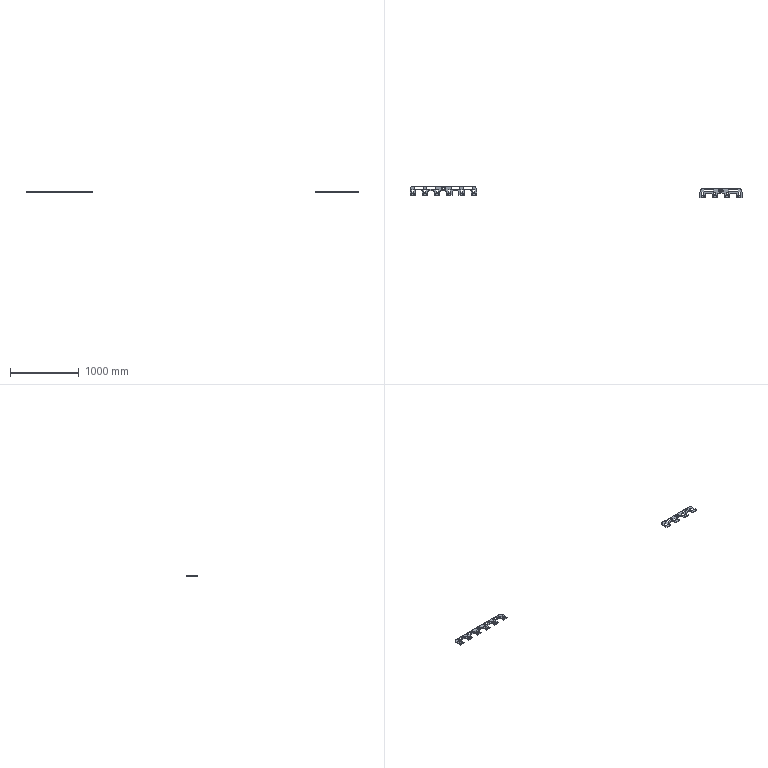NC program | NX | posted with a generic post | part box 4825 x 168.213 x 13 mm
Lines 1366 to 2532 of 4378:
(ZLEVEL_PROFILE_COPY_1_COPY_COPY , TOOL : D6)
N2688 T06 M6
N2690 G54
N2692 G17 G0 G90 X414.221 Y-3.8 S9500 M3
N2694 G43 Z30. H6
N2696 Z-0.591
N2698 G94 G1 Y-4.997 F1000.
N2700 X414.284 Y-5.
N2702 X416.5 F1650.
N2704 Y-2.784
N2706 X416.497 Y-2.721
N2708 X415.3
N2710 G0 X414.221 Y-3.8 Z-1.182
N2712 G1 Y-4.997 F1000.
N2714 X414.284 Y-5.
N2716 X416.5 F1650.
N2718 Y-2.784
N2720 X416.497 Y-2.721
N2722 X415.3
N2724 G0 X414.221 Y-3.8 Z-1.773
N2726 G1 Y-4.997 F1000.
N2728 X414.284 Y-5.
N2730 X416.5 F1650.
N2732 Y-2.784
N2734 X416.497 Y-2.721
N2736 X415.3
N2738 G0 X414.221 Y-3.8 Z-2.364
N2740 G1 Y-4.997 F1000.
N2742 X414.284 Y-5.
N2744 X416.5 F1650.
N2746 Y-2.784
N2748 X416.497 Y-2.721
N2750 X415.3
N2752 G0 X414.221 Y-3.8 Z-2.955
N2754 G1 Y-4.997 F1000.
N2756 X414.284 Y-5.
N2758 X416.5 F1650.
N2760 Y-2.784
N2762 X416.497 Y-2.721
N2764 X415.3
N2766 G0 X414.221 Y-3.8 Z-3.545
N2768 G1 Y-4.997 F1000.
N2770 X414.284 Y-5.
N2772 X416.5 F1650.
N2774 Y-2.784
N2776 X416.497 Y-2.721
N2778 X415.3
N2780 G0 X414.221 Y-3.8 Z-4.136
N2782 G1 Y-4.997 F1000.
N2784 X414.284 Y-5.
N2786 X416.5 F1650.
N2788 Y-2.784
N2790 X416.497 Y-2.721
N2792 X415.3
N2794 G0 X414.221 Y-3.8 Z-4.727
N2796 G1 Y-4.997 F1000.
N2798 X414.284 Y-5.
N2800 X416.5 F1650.
N2802 Y-2.784
N2804 X416.497 Y-2.721
N2806 X415.3
N2808 G0 X414.221 Y-3.8 Z-5.318
N2810 G1 Y-4.997 F1000.
N2812 X414.284 Y-5.
N2814 X416.5 F1650.
N2816 Y-2.784
N2818 X416.497 Y-2.721
N2820 X415.3
N2822 G0 X414.221 Y-3.8 Z-5.909
N2824 G1 Y-4.997 F1000.
N2826 X414.284 Y-5.
N2828 X416.5 F1650.
N2830 Y-2.784
N2832 X416.497 Y-2.721
N2834 X415.3
N2836 G0 X414.221 Y-3.8 Z-6.5
N2838 G1 Y-4.997 F1000.
N2840 X414.284 Y-5.
N2842 X416.5 F1650.
N2844 Y-2.784
N2846 X416.497 Y-2.721
N2848 X415.3
N2850 G0 X414.221 Y-3.8 Z-7.091
N2852 G1 Y-4.997 F1000.
N2854 X414.284 Y-5.
N2856 X416.5 F1650.
N2858 Y-2.784
N2860 X416.497 Y-2.721
N2862 X415.3
N2864 G0 X414.221 Y-3.8 Z-7.682
N2866 G1 Y-4.997 F1000.
N2868 X414.284 Y-5.
N2870 X416.5 F1650.
N2872 Y-2.784
N2874 X416.497 Y-2.721
N2876 X415.3
N2878 G0 X414.211 Y-3.8 Z-8.273
N2880 G1 Y-4.997 F1000.
N2882 X414.273 Y-5.
N2884 X416.5 F1650.
N2886 Y-2.782
N2888 X416.497 Y-2.719
N2890 X415.3
N2892 G0 X414.211 Y-3.8 Z-8.864
N2894 G1 Y-4.997 F1000.
N2896 X414.273 Y-5.
N2898 X416.5 F1650.
N2900 Y-2.782
N2902 X416.497 Y-2.719
N2904 X415.3
N2906 G0 X414.211 Y-3.8 Z-9.455
N2908 G1 Y-4.997 F1000.
N2910 X414.273 Y-5.
N2912 X416.5 F1650.
N2914 Y-2.782
N2916 X416.497 Y-2.719
N2918 X415.3
N2920 G0 X414.211 Y-3.8 Z-10.045
N2922 G1 Y-4.997 F1000.
N2924 X414.273 Y-5.
N2926 X416.5 F1650.
N2928 Y-2.782
N2930 X416.497 Y-2.719
N2932 X415.3
N2934 G0 X414.211 Y-3.8 Z-10.636
N2936 G1 Y-4.997 F1000.
N2938 X414.273 Y-5.
N2940 X416.5 F1650.
N2942 Y-2.782
N2944 X416.497 Y-2.719
N2946 X415.3
N2948 G0 X414.211 Y-3.8 Z-11.227
N2950 G1 Y-4.997 F1000.
N2952 X414.273 Y-5.
N2954 X416.5 F1650.
N2956 Y-2.782
N2958 X416.497 Y-2.719
N2960 X415.3
N2962 G0 X414.211 Y-3.8 Z-11.818
N2964 G1 Y-4.997 F1000.
N2966 X414.273 Y-5.
N2968 X416.5 F1650.
N2970 Y-2.782
N2972 X416.497 Y-2.719
N2974 X415.3
N2976 G0 X414.211 Y-3.8 Z-12.409
N2978 G1 Y-4.997 F1000.
N2980 X414.273 Y-5.
N2982 X416.5 F1650.
N2984 Y-2.782
N2986 X416.497 Y-2.719
N2988 X415.3
N2990 G0 X414.211 Y-3.8 Z-13.
N2992 G1 Y-4.997 F1000.
N2994 X414.273 Y-5.
N2996 X416.5 F1650.
N2998 Y-2.782
N3000 X416.497 Y-2.719
N3002 X415.3
N3004 G0 Z30.
N3006 Y18.721
N3008 Z-0.591
N3010 G1 X416.497 F1000.
N3012 X416.5 Y18.784
N3014 Y21. F1650.
N3016 X414.284
N3018 X414.221 Y20.997
N3020 Y19.8
N3022 G0 X415.3 Y18.721 Z-1.182
N3024 G1 X416.497 F1000.
N3026 X416.5 Y18.784
N3028 Y21. F1650.
N3030 X414.284
N3032 X414.221 Y20.997
N3034 Y19.8
N3036 G0 X415.3 Y18.721 Z-1.773
N3038 G1 X416.497 F1000.
N3040 X416.5 Y18.784
N3042 Y21. F1650.
N3044 X414.284
N3046 X414.221 Y20.997
N3048 Y19.8
N3050 G0 X415.3 Y18.721 Z-2.364
N3052 G1 X416.497 F1000.
N3054 X416.5 Y18.784
N3056 Y21. F1650.
N3058 X414.284
N3060 X414.221 Y20.997
N3062 Y19.8
N3064 G0 X415.3 Y18.721 Z-2.955
N3066 G1 X416.497 F1000.
N3068 X416.5 Y18.784
N3070 Y21. F1650.
N3072 X414.284
N3074 X414.221 Y20.997
N3076 Y19.8
N3078 G0 X415.3 Y18.721 Z-3.545
N3080 G1 X416.497 F1000.
N3082 X416.5 Y18.784
N3084 Y21. F1650.
N3086 X414.284
N3088 X414.221 Y20.997
N3090 Y19.8
N3092 G0 X415.3 Y18.721 Z-4.136
N3094 G1 X416.497 F1000.
N3096 X416.5 Y18.784
N3098 Y21. F1650.
N3100 X414.284
N3102 X414.221 Y20.997
N3104 Y19.8
N3106 G0 X415.3 Y18.721 Z-4.727
N3108 G1 X416.497 F1000.
N3110 X416.5 Y18.784
N3112 Y21. F1650.
N3114 X414.284
N3116 X414.221 Y20.997
N3118 Y19.8
N3120 G0 X415.3 Y18.721 Z-5.318
N3122 G1 X416.497 F1000.
N3124 X416.5 Y18.784
N3126 Y21. F1650.
N3128 X414.284
N3130 X414.221 Y20.997
N3132 Y19.8
N3134 G0 X415.3 Y18.721 Z-5.909
N3136 G1 X416.497 F1000.
N3138 X416.5 Y18.784
N3140 Y21. F1650.
N3142 X414.284
N3144 X414.221 Y20.997
N3146 Y19.8
N3148 G0 X415.3 Y18.721 Z-6.5
N3150 G1 X416.497 F1000.
N3152 X416.5 Y18.784
N3154 Y21. F1650.
N3156 X414.284
N3158 X414.221 Y20.997
N3160 Y19.8
N3162 G0 X415.3 Y18.721 Z-7.091
N3164 G1 X416.497 F1000.
N3166 X416.5 Y18.784
N3168 Y21. F1650.
N3170 X414.284
N3172 X414.221 Y20.997
N3174 Y19.8
N3176 G0 X415.3 Y18.721 Z-7.682
N3178 G1 X416.497 F1000.
N3180 X416.5 Y18.784
N3182 Y21. F1650.
N3184 X414.284
N3186 X414.221 Y20.997
N3188 Y19.8
N3190 G0 X415.3 Y18.729 Z-8.273
N3192 G1 X416.497 F1000.
N3194 X416.5 Y18.792
N3196 Y20.988 F1650.
N3198 Y21.
N3200 X414.292
N3202 X414.229 Y20.997
N3204 Y19.8
N3206 G0 X415.3 Y18.729 Z-8.864
N3208 G1 X416.497 F1000.
N3210 X416.5 Y18.792
N3212 Y20.988 F1650.
N3214 Y21.
N3216 X414.292
N3218 X414.229 Y20.997
N3220 Y19.8
N3222 G0 X415.3 Y18.729 Z-9.455
N3224 G1 X416.497 F1000.
N3226 X416.5 Y18.792
N3228 Y20.988 F1650.
N3230 Y21.
N3232 X414.292
N3234 X414.229 Y20.997
N3236 Y19.8
N3238 G0 X415.3 Y18.729 Z-10.045
N3240 G1 X416.497 F1000.
N3242 X416.5 Y18.792
N3244 Y20.988 F1650.
N3246 Y21.
N3248 X414.292
N3250 X414.229 Y20.997
N3252 Y19.8
N3254 G0 X415.3 Y18.729 Z-10.636
N3256 G1 X416.497 F1000.
N3258 X416.5 Y18.792
N3260 Y20.988 F1650.
N3262 Y21.
N3264 X414.292
N3266 X414.229 Y20.997
N3268 Y19.8
N3270 G0 X415.3 Y18.729 Z-11.227
N3272 G1 X416.497 F1000.
N3274 X416.5 Y18.792
N3276 Y20.988 F1650.
N3278 Y21.
N3280 X414.292
N3282 X414.229 Y20.997
N3284 Y19.8
N3286 G0 X415.3 Y18.729 Z-11.818
N3288 G1 X416.497 F1000.
N3290 X416.5 Y18.792
N3292 Y20.988 F1650.
N3294 Y21.
N3296 X414.292
N3298 X414.229 Y20.997
N3300 Y19.8
N3302 G0 X415.3 Y18.729 Z-12.409
N3304 G1 X416.497 F1000.
N3306 X416.5 Y18.792
N3308 Y20.988 F1650.
N3310 Y21.
N3312 X414.292
N3314 X414.229 Y20.997
N3316 Y19.8
N3318 G0 X415.3 Y18.729 Z-13.
N3320 G1 X416.497 F1000.
N3322 X416.5 Y18.792
N3324 Y20.988 F1650.
N3326 Y21.
N3328 X414.292
N3330 X414.229 Y20.997
N3332 Y19.8
N3334 G0 Z30.
N3336 X296.979
N3338 Z-0.591
N3340 G1 Y20.997 F1000.
N3342 X296.916 Y21.
N3344 X294.7 F1650.
N3346 Y18.784
N3348 X294.703 Y18.721
N3350 X295.9
N3352 G0 X296.979 Y19.8 Z-1.182
N3354 G1 Y20.997 F1000.
N3356 X296.916 Y21.
N3358 X294.7 F1650.
N3360 Y18.784
N3362 X294.703 Y18.721
N3364 X295.9
N3366 G0 X296.979 Y19.8 Z-1.773
N3368 G1 Y20.997 F1000.
N3370 X296.916 Y21.
N3372 X294.7 F1650.
N3374 Y18.784
N3376 X294.703 Y18.721
N3378 X295.9
N3380 G0 X296.979 Y19.8 Z-2.364
N3382 G1 Y20.997 F1000.
N3384 X296.916 Y21.
N3386 X294.7 F1650.
N3388 Y18.784
N3390 X294.703 Y18.721
N3392 X295.9
N3394 G0 X296.979 Y19.8 Z-2.955
N3396 G1 Y20.997 F1000.
N3398 X296.916 Y21.
N3400 X294.7 F1650.
N3402 Y18.784
N3404 X294.703 Y18.721
N3406 X295.9
N3408 G0 X296.979 Y19.8 Z-3.545
N3410 G1 Y20.997 F1000.
N3412 X296.916 Y21.
N3414 X294.7 F1650.
N3416 Y18.784
N3418 X294.703 Y18.721
N3420 X295.9
N3422 G0 X296.979 Y19.8 Z-4.136
N3424 G1 Y20.997 F1000.
N3426 X296.916 Y21.
N3428 X294.7 F1650.
N3430 Y18.784
N3432 X294.703 Y18.721
N3434 X295.9
N3436 G0 X296.979 Y19.8 Z-4.727
N3438 G1 Y20.997 F1000.
N3440 X296.916 Y21.
N3442 X294.7 F1650.
N3444 Y18.784
N3446 X294.703 Y18.721
N3448 X295.9
N3450 G0 X296.979 Y19.8 Z-5.318
N3452 G1 Y20.997 F1000.
N3454 X296.916 Y21.
N3456 X294.7 F1650.
N3458 Y18.784
N3460 X294.703 Y18.721
N3462 X295.9
N3464 G0 X296.979 Y19.8 Z-5.909
N3466 G1 Y20.997 F1000.
N3468 X296.916 Y21.
N3470 X294.7 F1650.
N3472 Y18.784
N3474 X294.703 Y18.721
N3476 X295.9
N3478 G0 X296.979 Y19.8 Z-6.5
N3480 G1 Y20.997 F1000.
N3482 X296.916 Y21.
N3484 X294.7 F1650.
N3486 Y18.784
N3488 X294.703 Y18.721
N3490 X295.9
N3492 G0 X296.979 Y19.8 Z-7.091
N3494 G1 Y20.997 F1000.
N3496 X296.916 Y21.
N3498 X294.7 F1650.
N3500 Y18.784
N3502 X294.703 Y18.721
N3504 X295.9
N3506 G0 X296.979 Y19.8 Z-7.682
N3508 G1 Y20.997 F1000.
N3510 X296.916 Y21.
N3512 X294.7 F1650.
N3514 Y18.784
N3516 X294.703 Y18.721
N3518 X295.9
N3520 G0 X296.97 Y19.8 Z-8.273
N3522 G1 Y20.997 F1000.
N3524 X296.907 Y21.
N3526 X294.7 F1650.
N3528 Y18.785
N3530 X294.703 Y18.722
N3532 X295.9
N3534 G0 X296.97 Y19.8 Z-8.864
N3536 G1 Y20.997 F1000.
N3538 X296.907 Y21.
N3540 X294.7 F1650.
N3542 Y18.785
N3544 X294.703 Y18.722
N3546 X295.9
N3548 G0 X296.97 Y19.8 Z-9.455
N3550 G1 Y20.997 F1000.
N3552 X296.907 Y21.
N3554 X294.7 F1650.
N3556 Y18.785
N3558 X294.703 Y18.722
N3560 X295.9
N3562 G0 X296.97 Y19.8 Z-10.045
N3564 G1 Y20.997 F1000.
N3566 X296.907 Y21.
N3568 X294.7 F1650.
N3570 Y18.785
N3572 X294.703 Y18.722
N3574 X295.9
N3576 G0 X296.97 Y19.8 Z-10.636
N3578 G1 Y20.997 F1000.
N3580 X296.907 Y21.
N3582 X294.7 F1650.
N3584 Y18.785
N3586 X294.703 Y18.722
N3588 X295.9
N3590 G0 X296.97 Y19.8 Z-11.227
N3592 G1 Y20.997 F1000.
N3594 X296.907 Y21.
N3596 X294.7 F1650.
N3598 Y18.785
N3600 X294.703 Y18.722
N3602 X295.9
N3604 G0 X296.97 Y19.8 Z-11.818
N3606 G1 Y20.997 F1000.
N3608 X296.907 Y21.
N3610 X294.7 F1650.
N3612 Y18.785
N3614 X294.703 Y18.722
N3616 X295.9
N3618 G0 X296.97 Y19.8 Z-12.409
N3620 G1 Y20.997 F1000.
N3622 X296.907 Y21.
N3624 X294.7 F1650.
N3626 Y18.785
N3628 X294.703 Y18.722
N3630 X295.9
N3632 G0 X296.97 Y19.8 Z-13.
N3634 G1 Y20.997 F1000.
N3636 X296.907 Y21.
N3638 X294.7 F1650.
N3640 Y18.785
N3642 X294.703 Y18.722
N3644 X295.9
N3646 G0 Z30.
N3648 Y-2.721
N3650 Z-0.591
N3652 G1 X294.703 F1000.
N3654 X294.7 Y-2.784
N3656 Y-4.947 F1650.
N3658 X294.699 Y-5.001
N3660 X296.916 Y-5.
N3662 X296.979 Y-4.997
N3664 Y-3.8
N3666 G0 X295.9 Y-2.721 Z-1.182
N3668 G1 X294.703 F1000.
N3670 X294.7 Y-2.784
N3672 Y-4.947 F1650.
N3674 X294.699 Y-5.001
N3676 X296.916 Y-5.
N3678 X296.979 Y-4.997
N3680 Y-3.8
N3682 G0 X295.9 Y-2.721 Z-1.773
N3684 G1 X294.703 F1000.
N3686 X294.7 Y-2.784
N3688 Y-4.947 F1650.
N3690 X294.699 Y-5.001
N3692 X296.916 Y-5.
N3694 X296.979 Y-4.997
N3696 Y-3.8
N3698 G0 X295.9 Y-2.721 Z-2.364
N3700 G1 X294.703 F1000.
N3702 X294.7 Y-2.784
N3704 Y-4.947 F1650.
N3706 Y-5.
N3708 X296.916
N3710 X296.979 Y-4.997
N3712 Y-3.8
N3714 G0 X295.9 Y-2.721 Z-2.955
N3716 G1 X294.703 F1000.
N3718 X294.7 Y-2.784
N3720 Y-4.947 F1650.
N3722 Y-5.
N3724 X296.916
N3726 X296.979 Y-4.997
N3728 Y-3.8
N3730 G0 X295.9 Y-2.721 Z-3.545
N3732 G1 X294.703 F1000.
N3734 X294.7 Y-2.784
N3736 Y-4.947 F1650.
N3738 Y-5.
N3740 X296.916
N3742 X296.979 Y-4.997
N3744 Y-3.8
N3746 G0 X295.9 Y-2.721 Z-4.136
N3748 G1 X294.703 F1000.
N3750 X294.7 Y-2.784
N3752 Y-4.947 F1650.
N3754 Y-5.
N3756 X296.916
N3758 X296.979 Y-4.997
N3760 Y-3.8
N3762 G0 X295.9 Y-2.721 Z-4.727
N3764 G1 X294.703 F1000.
N3766 X294.7 Y-2.784
N3768 Y-5. F1650.
N3770 X296.916
N3772 X296.979 Y-4.997
N3774 Y-3.8
N3776 G0 X295.9 Y-2.721 Z-5.318
N3778 G1 X294.703 F1000.
N3780 X294.7 Y-2.784
N3782 Y-5. F1650.
N3784 X296.916
N3786 X296.979 Y-4.997
N3788 Y-3.8
N3790 G0 X295.9 Y-2.721 Z-5.909
N3792 G1 X294.703 F1000.
N3794 X294.7 Y-2.784
N3796 Y-4.961 F1650.
N3798 Y-5.
N3800 X296.916
N3802 X296.979 Y-4.997
N3804 Y-3.8
N3806 G0 X295.9 Y-2.721 Z-6.5
N3808 G1 X294.703 F1000.
N3810 X294.7 Y-2.784
N3812 Y-4.961 F1650.
N3814 Y-5.
N3816 X296.916
N3818 X296.979 Y-4.997
N3820 Y-3.8
N3822 G0 X295.9 Y-2.721 Z-7.091
N3824 G1 X294.703 F1000.
N3826 X294.7 Y-2.784
N3828 Y-4.961 F1650.
N3830 X294.701 Y-5.
N3832 X296.916
N3834 X296.979 Y-4.997
N3836 Y-3.8
N3838 G0 X295.9 Y-2.721 Z-7.682
N3840 G1 X294.703 F1000.
N3842 X294.7 Y-2.784
N3844 Y-4.961 F1650.
N3846 X294.701 Y-5.
N3848 X296.916
N3850 X296.979 Y-4.997
N3852 Y-3.8
N3854 G0 X295.9 Y-2.721 Z-8.273
N3856 G1 X294.703 F1000.
N3858 X294.7 Y-2.784
N3860 Y-5. F1650.
N3862 X296.916
N3864 X296.979 Y-4.997
N3866 Y-3.8
N3868 G0 X295.9 Y-2.721 Z-8.864
N3870 G1 X294.703 F1000.
N3872 X294.7 Y-2.784
N3874 Y-5. F1650.
N3876 X296.916
N3878 X296.979 Y-4.997
N3880 Y-3.8
N3882 G0 X295.9 Y-2.721 Z-9.455
N3884 G1 X294.703 F1000.
N3886 X294.7 Y-2.784
N3888 Y-5. F1650.
N3890 X296.916
N3892 X296.979 Y-4.997
N3894 Y-3.8
N3896 G0 X295.9 Y-2.721 Z-10.045
N3898 G1 X294.703 F1000.
N3900 X294.7 Y-2.784
N3902 Y-5. F1650.
N3904 X296.916
N3906 X296.979 Y-4.997
N3908 Y-3.8
N3910 G0 X295.9 Y-2.721 Z-10.636
N3912 G1 X294.703 F1000.
N3914 X294.7 Y-2.784
N3916 Y-5. F1650.
N3918 X296.916
N3920 X296.979 Y-4.997
N3922 Y-3.8
N3924 G0 X295.9 Y-2.721 Z-11.227
N3926 G1 X294.703 F1000.
N3928 X294.7 Y-2.784
N3930 Y-5. F1650.
N3932 X296.916
N3934 X296.979 Y-4.997
N3936 Y-3.8
N3938 G0 X295.9 Y-2.721 Z-11.818
N3940 G1 X294.703 F1000.
N3942 X294.7 Y-2.784
N3944 Y-5. F1650.
N3946 X296.916
N3948 X296.979 Y-4.997
N3950 Y-3.8
N3952 G0 X295.9 Y-2.721 Z-12.409
N3954 G1 X294.703 F1000.
N3956 X294.7 Y-2.784
N3958 Y-5. F1650.
N3960 X296.916
N3962 X296.979 Y-4.997
N3964 Y-3.8
N3966 G0 X295.9 Y-2.721 Z-13.
N3968 G1 X294.703 F1000.
N3970 X294.7 Y-2.784
N3972 Y-5. F1650.
N3974 X296.916
N3976 X296.979 Y-4.997
N3978 Y-3.8
N3980 G0 Z30.
N3982 X236.421
N3984 Z-0.591
N3986 G1 Y-4.997 F1000.
N3988 X236.484 Y-5.
N3990 X238.7 F1650.
N3992 Y-2.784
N3994 X238.697 Y-2.721
N3996 X237.5
N3998 G0 X236.421 Y-3.8 Z-1.182
N4000 G1 Y-4.997 F1000.
N4002 X236.484 Y-5.
N4004 X238.7 F1650.
N4006 Y-2.784
N4008 X238.697 Y-2.721
N4010 X237.5
N4012 G0 X236.421 Y-3.8 Z-1.773
N4014 G1 Y-4.997 F1000.
N4016 X236.484 Y-5.
N4018 X238.7 F1650.
N4020 Y-2.784
N4022 X238.697 Y-2.721
N4024 X237.5
N4026 G0 X236.421 Y-3.8 Z-2.364
N4028 G1 Y-4.997 F1000.
N4030 X236.484 Y-5.
N4032 X238.7 F1650.
N4034 Y-2.784
N4036 X238.697 Y-2.721
N4038 X237.5
N4040 G0 X236.421 Y-3.8 Z-2.955
N4042 G1 Y-4.997 F1000.
N4044 X236.484 Y-5.
N4046 X238.7 F1650.
N4048 Y-2.784
N4050 X238.697 Y-2.721
N4052 X237.5
N4054 G0 X236.421 Y-3.8 Z-3.545
N4056 G1 Y-4.997 F1000.
N4058 X236.484 Y-5.
N4060 X238.7 F1650.
N4062 Y-2.784
N4064 X238.697 Y-2.721
N4066 X237.5
N4068 G0 X236.421 Y-3.8 Z-4.136
N4070 G1 Y-4.997 F1000.
N4072 X236.484 Y-5.
N4074 X238.7 F1650.
N4076 Y-2.784
N4078 X238.697 Y-2.721
N4080 X237.5
N4082 G0 X236.421 Y-3.8 Z-4.727
N4084 G1 Y-4.997 F1000.
N4086 X236.484 Y-5.
N4088 X238.7 F1650.
N4090 Y-2.784
N4092 X238.697 Y-2.721
N4094 X237.5
N4096 G0 X236.421 Y-3.8 Z-5.318
N4098 G1 Y-4.997 F1000.
N4100 X236.484 Y-5.
N4102 X238.7 F1650.
N4104 Y-2.784
N4106 X238.697 Y-2.721
N4108 X237.5
N4110 G0 X236.421 Y-3.8 Z-5.909
N4112 G1 Y-4.997 F1000.
N4114 X236.484 Y-5.
N4116 X238.7 F1650.
N4118 Y-2.784
N4120 X238.697 Y-2.721
N4122 X237.5
N4124 G0 X236.421 Y-3.8 Z-6.5
N4126 G1 Y-4.997 F1000.
N4128 X236.484 Y-5.
N4130 X238.7 F1650.
N4132 Y-2.784
N4134 X238.697 Y-2.721
N4136 X237.5
N4138 G0 X236.421 Y-3.8 Z-7.091
N4140 G1 Y-4.997 F1000.
N4142 X236.484 Y-5.
N4144 X238.7 F1650.
N4146 Y-2.784
N4148 X238.697 Y-2.721
N4150 X237.5
N4152 G0 X236.421 Y-3.8 Z-7.682
N4154 G1 Y-4.997 F1000.
N4156 X236.484 Y-5.
N4158 X238.7 F1650.
N4160 Y-2.784
N4162 X238.697 Y-2.721
N4164 X237.5
N4166 G0 X236.409 Y-3.8 Z-8.273
N4168 G1 Y-4.997 F1000.
N4170 X236.472 Y-5.
N4172 X238.7 F1650.
N4174 Y-2.781
N4176 X238.697 Y-2.719
N4178 X237.5
N4180 G0 X236.409 Y-3.8 Z-8.864
N4182 G1 Y-4.997 F1000.
N4184 X236.472 Y-5.
N4186 X238.7 F1650.
N4188 Y-2.781
N4190 X238.697 Y-2.719
N4192 X237.5
N4194 G0 X236.409 Y-3.8 Z-9.455
N4196 G1 Y-4.997 F1000.
N4198 X236.472 Y-5.
N4200 X238.7 F1650.
N4202 Y-2.781
N4204 X238.697 Y-2.719
N4206 X237.5
N4208 G0 X236.409 Y-3.8 Z-10.045
N4210 G1 Y-4.997 F1000.
N4212 X236.472 Y-5.
N4214 X238.7 F1650.
N4216 Y-2.781
N4218 X238.697 Y-2.719
N4220 X237.5
N4222 G0 X236.409 Y-3.8 Z-10.636
N4224 G1 Y-4.997 F1000.
N4226 X236.472 Y-5.
N4228 X238.7 F1650.
N4230 Y-2.781
N4232 X238.697 Y-2.719
N4234 X237.5
N4236 G0 X236.409 Y-3.8 Z-11.227
N4238 G1 Y-4.997 F1000.
N4240 X236.472 Y-5.
N4242 X238.7 F1650.
N4244 Y-2.781
N4246 X238.697 Y-2.719
N4248 X237.5
N4250 G0 X236.409 Y-3.8 Z-11.818
N4252 G1 Y-4.997 F1000.
N4254 X236.472 Y-5.
N4256 X238.7 F1650.
N4258 Y-2.781
N4260 X238.697 Y-2.719
N4262 X237.5
N4264 G0 X236.409 Y-3.8 Z-12.409
N4266 G1 Y-4.997 F1000.
N4268 X236.472 Y-5.
N4270 X238.7 F1650.
N4272 Y-2.781
N4274 X238.697 Y-2.719
N4276 X237.5
N4278 G0 X236.409 Y-3.8 Z-13.
N4280 G1 Y-4.997 F1000.
N4282 X236.472 Y-5.
N4284 X238.7 F1650.
N4286 Y-2.781
N4288 X238.697 Y-2.719
N4290 X237.5
N4292 G0 Z30.
N4294 Y18.721
N4296 Z-0.591
N4298 G1 X238.697 F1000.
N4300 X238.7 Y18.784
N4302 Y21. F1650.
N4304 X236.484
N4306 X236.421 Y20.997
N4308 Y19.8
N4310 G0 X237.5 Y18.721 Z-1.182
N4312 G1 X238.697 F1000.
N4314 X238.7 Y18.784
N4316 Y21. F1650.
N4318 X236.484
N4320 X236.421 Y20.997
N4322 Y19.8
N4324 G0 X237.5 Y18.721 Z-1.773
N4326 G1 X238.697 F1000.
N4328 X238.7 Y18.784
N4330 Y21. F1650.
N4332 X236.484
N4334 X236.421 Y20.997
N4336 Y19.8
N4338 G0 X237.5 Y18.721 Z-2.364
N4340 G1 X238.697 F1000.
N4342 X238.7 Y18.784
N4344 Y21. F1650.
N4346 X236.484
N4348 X236.421 Y20.997
N4350 Y19.8
N4352 G0 X237.5 Y18.721 Z-2.955
N4354 G1 X238.697 F1000.
N4356 X238.7 Y18.784
N4358 Y21. F1650.
N4360 X236.484
N4362 X236.421 Y20.997
N4364 Y19.8
N4366 G0 X237.5 Y18.721 Z-3.545
N4368 G1 X238.697 F1000.
N4370 X238.7 Y18.784
N4372 Y21. F1650.
N4374 X236.484
N4376 X236.421 Y20.997
N4378 Y19.8
N4380 G0 X237.5 Y18.721 Z-4.136
N4382 G1 X238.697 F1000.
N4384 X238.7 Y18.784
N4386 Y21. F1650.
N4388 X236.484
N4390 X236.421 Y20.997
N4392 Y19.8
N4394 G0 X237.5 Y18.721 Z-4.727
N4396 G1 X238.697 F1000.
N4398 X238.7 Y18.784
N4400 Y21. F1650.
N4402 X236.484
N4404 X236.421 Y20.997
N4406 Y19.8
N4408 G0 X237.5 Y18.721 Z-5.318
N4410 G1 X238.697 F1000.
N4412 X238.7 Y18.784
N4414 Y21. F1650.
N4416 X236.484
N4418 X236.421 Y20.997
N4420 Y19.8
N4422 G0 X237.5 Y18.721 Z-5.909
N4424 G1 X238.697 F1000.
N4426 X238.7 Y18.784
N4428 Y21. F1650.
N4430 X236.484
N4432 X236.421 Y20.997
N4434 Y19.8
N4436 G0 X237.5 Y18.721 Z-6.5
N4438 G1 X238.697 F1000.
N4440 X238.7 Y18.784
N4442 Y21. F1650.
N4444 X236.484
N4446 X236.421 Y20.997
N4448 Y19.8
N4450 G0 X237.5 Y18.721 Z-7.091
N4452 G1 X238.697 F1000.
N4454 X238.7 Y18.784
N4456 Y21. F1650.
N4458 X236.484
N4460 X236.421 Y20.997
N4462 Y19.8
N4464 G0 X237.5 Y18.721 Z-7.682
N4466 G1 X238.697 F1000.
N4468 X238.7 Y18.784
N4470 Y21. F1650.
N4472 X236.484
N4474 X236.421 Y20.997
N4476 Y19.8
N4478 G0 X237.5 Y18.73 Z-8.273
N4480 G1 X238.697 F1000.
N4482 X238.7 Y18.793
N4484 Y20.988 F1650.
N4486 Y21.
N4488 X236.488
N4490 X236.425 Y20.997
N4492 Y19.8
N4494 G0 X237.5 Y18.73 Z-8.864
N4496 G1 X238.697 F1000.
N4498 X238.7 Y18.793
N4500 Y20.988 F1650.
N4502 Y21.
N4504 X236.488
N4506 X236.425 Y20.997
N4508 Y19.8
N4510 G0 X237.5 Y18.73 Z-9.455
N4512 G1 X238.697 F1000.
N4514 X238.7 Y18.793
N4516 Y20.988 F1650.
N4518 Y21.
N4520 X236.488
N4522 X236.425 Y20.997
N4524 Y19.8
N4526 G0 X237.5 Y18.73 Z-10.045
N4528 G1 X238.697 F1000.
N4530 X238.7 Y18.793
N4532 Y20.988 F1650.
N4534 Y21.
N4536 X236.488
N4538 X236.425 Y20.997
N4540 Y19.8
N4542 G0 X237.5 Y18.73 Z-10.636
N4544 G1 X238.697 F1000.
N4546 X238.7 Y18.793
N4548 Y20.988 F1650.
N4550 Y21.
N4552 X236.488
N4554 X236.425 Y20.997
N4556 Y19.8
N4558 G0 X237.5 Y18.73 Z-11.227
N4560 G1 X238.697 F1000.
N4562 X238.7 Y18.793
N4564 Y20.988 F1650.
N4566 Y21.
N4568 X236.488
N4570 X236.425 Y20.997
N4572 Y19.8
N4574 G0 X237.5 Y18.73 Z-11.818
N4576 G1 X238.697 F1000.
N4578 X238.7 Y18.793
N4580 Y20.988 F1650.
N4582 Y21.
N4584 X236.488
N4586 X236.425 Y20.997
N4588 Y19.8
N4590 G0 X237.5 Y18.73 Z-12.409
N4592 G1 X238.697 F1000.
N4594 X238.7 Y18.793
N4596 Y20.988 F1650.
N4598 Y21.
N4600 X236.488
N4602 X236.425 Y20.997
N4604 Y19.8
N4606 G0 X237.5 Y18.73 Z-13.
N4608 G1 X238.697 F1000.
N4610 X238.7 Y18.793
N4612 Y20.988 F1650.
N4614 Y21.
N4616 X236.488
N4618 X236.425 Y20.997
N4620 Y19.8
N4622 G0 Z30.
N4624 X119.179
N4626 Z-0.591
N4628 G1 Y20.997 F1000.
N4630 X119.116 Y21.
N4632 X116.9 F1650.
N4634 Y18.784
N4636 X116.903 Y18.721
N4638 X118.1
N4640 G0 X119.179 Y19.8 Z-1.182
N4642 G1 Y20.997 F1000.
N4644 X119.116 Y21.
N4646 X116.9 F1650.
N4648 Y18.784
N4650 X116.903 Y18.721
N4652 X118.1
N4654 G0 X119.179 Y19.8 Z-1.773
N4656 G1 Y20.997 F1000.
N4658 X119.116 Y21.
N4660 X116.9 F1650.
N4662 Y18.784
N4664 X116.903 Y18.721
N4666 X118.1
N4668 G0 X119.179 Y19.8 Z-2.364
N4670 G1 Y20.997 F1000.
N4672 X119.116 Y21.
N4674 X116.9 F1650.
N4676 Y18.784
N4678 X116.903 Y18.721
N4680 X118.1
N4682 G0 X119.179 Y19.8 Z-2.955
N4684 G1 Y20.997 F1000.
N4686 X119.116 Y21.
N4688 X116.9 F1650.
N4690 Y18.784
N4692 X116.903 Y18.721
N4694 X118.1
N4696 G0 X119.179 Y19.8 Z-3.545
N4698 G1 Y20.997 F1000.
N4700 X119.116 Y21.
N4702 X116.9 F1650.
N4704 Y18.784
N4706 X116.903 Y18.721
N4708 X118.1
N4710 G0 X119.179 Y19.8 Z-4.136
N4712 G1 Y20.997 F1000.
N4714 X119.116 Y21.
N4716 X116.9 F1650.
N4718 Y18.784
N4720 X116.903 Y18.721
N4722 X118.1
N4724 G0 X119.179 Y19.8 Z-4.727
N4726 G1 Y20.997 F1000.
N4728 X119.116 Y21.
N4730 X116.9 F1650.
N4732 Y18.784
N4734 X116.903 Y18.721
N4736 X118.1
N4738 G0 X119.179 Y19.8 Z-5.318
N4740 G1 Y20.997 F1000.
N4742 X119.116 Y21.
N4744 X116.9 F1650.
N4746 Y18.784
N4748 X116.903 Y18.721
N4750 X118.1
N4752 G0 X119.179 Y19.8 Z-5.909
N4754 G1 Y20.997 F1000.
N4756 X119.116 Y21.
N4758 X116.9 F1650.
N4760 Y18.784
N4762 X116.903 Y18.721
N4764 X118.1
N4766 G0 X119.179 Y19.8 Z-6.5
N4768 G1 Y20.997 F1000.
N4770 X119.116 Y21.
N4772 X116.9 F1650.
N4774 Y18.784
N4776 X116.903 Y18.721
N4778 X118.1
N4780 G0 X119.179 Y19.8 Z-7.091
N4782 G1 Y20.997 F1000.
N4784 X119.116 Y21.
N4786 X116.9 F1650.
N4788 Y18.784
N4790 X116.903 Y18.721
N4792 X118.1
N4794 G0 X119.179 Y19.8 Z-7.682
N4796 G1 Y20.997 F1000.
N4798 X119.116 Y21.
N4800 X116.9 F1650.
N4802 Y18.784
N4804 X116.903 Y18.721
N4806 X118.1
N4808 G0 X119.168 Y19.8 Z-8.273
N4810 G1 Y20.997 F1000.
N4812 X119.105 Y21.
N4814 X116.9 F1650.
N4816 Y18.787
N4818 X116.903 Y18.724
N4820 X118.1
N4822 G0 X119.168 Y19.8 Z-8.864
N4824 G1 Y20.997 F1000.
N4826 X119.105 Y21.
N4828 X116.9 F1650.
N4830 Y18.787
N4832 X116.903 Y18.724
N4834 X118.1
N4836 G0 X119.168 Y19.8 Z-9.455
N4838 G1 Y20.997 F1000.
N4840 X119.105 Y21.
N4842 X116.9 F1650.
N4844 Y18.787
N4846 X116.903 Y18.724
N4848 X118.1
N4850 G0 X119.168 Y19.8 Z-10.045
N4852 G1 Y20.997 F1000.
N4854 X119.105 Y21.
N4856 X116.9 F1650.
N4858 Y18.787
N4860 X116.903 Y18.724
N4862 X118.1
N4864 G0 X119.168 Y19.8 Z-10.636
N4866 G1 Y20.997 F1000.
N4868 X119.105 Y21.
N4870 X116.9 F1650.
N4872 Y18.787
N4874 X116.903 Y18.724
N4876 X118.1
N4878 G0 X119.168 Y19.8 Z-11.227
N4880 G1 Y20.997 F1000.
N4882 X119.105 Y21.
N4884 X116.9 F1650.
N4886 Y18.787
N4888 X116.903 Y18.724
N4890 X118.1
N4892 G0 X119.168 Y19.8 Z-11.818
N4894 G1 Y20.997 F1000.
N4896 X119.105 Y21.
N4898 X116.9 F1650.
N4900 Y18.787
N4902 X116.903 Y18.724
N4904 X118.1
N4906 G0 X119.168 Y19.8 Z-12.409
N4908 G1 Y20.997 F1000.
N4910 X119.105 Y21.
N4912 X116.9 F1650.
N4914 Y18.787
N4916 X116.903 Y18.724
N4918 X118.1
N4920 G0 X119.168 Y19.8 Z-13.
N4922 G1 Y20.997 F1000.
N4924 X119.105 Y21.
N4926 X116.9 F1650.
N4928 Y18.787
N4930 X116.903 Y18.724
N4932 X118.1
N4934 G0 Z30.
N4936 Y-2.721
N4938 Z-0.591
N4940 G1 X116.903 F1000.
N4942 X116.9 Y-2.784
N4944 Y-4.947 F1650.
N4946 X116.899 Y-5.001
N4948 X119.116 Y-5.
N4950 X119.179 Y-4.997
N4952 Y-3.8
N4954 G0 X118.1 Y-2.721 Z-1.182
N4956 G1 X116.903 F1000.
N4958 X116.9 Y-2.784
N4960 Y-4.947 F1650.
N4962 X116.899 Y-5.001
N4964 X119.116 Y-5.
N4966 X119.179 Y-4.997
N4968 Y-3.8
N4970 G0 X118.1 Y-2.721 Z-1.773
N4972 G1 X116.903 F1000.
N4974 X116.9 Y-2.784
N4976 Y-4.947 F1650.
N4978 X116.899 Y-5.001
N4980 X119.116 Y-5.
N4982 X119.179 Y-4.997
N4984 Y-3.8
N4986 G0 X118.1 Y-2.721 Z-2.364
N4988 G1 X116.903 F1000.
N4990 X116.9 Y-2.784
N4992 Y-4.947 F1650.
N4994 X116.899 Y-5.001
N4996 X119.116 Y-5.
N4998 X119.179 Y-4.997
N5000 Y-3.8
N5002 G0 X118.1 Y-2.721 Z-2.955
N5004 G1 X116.903 F1000.
N5006 X116.9 Y-2.784
N5008 Y-4.947 F1650.
N5010 Y-5.
N5012 X119.116
N5014 X119.179 Y-4.997